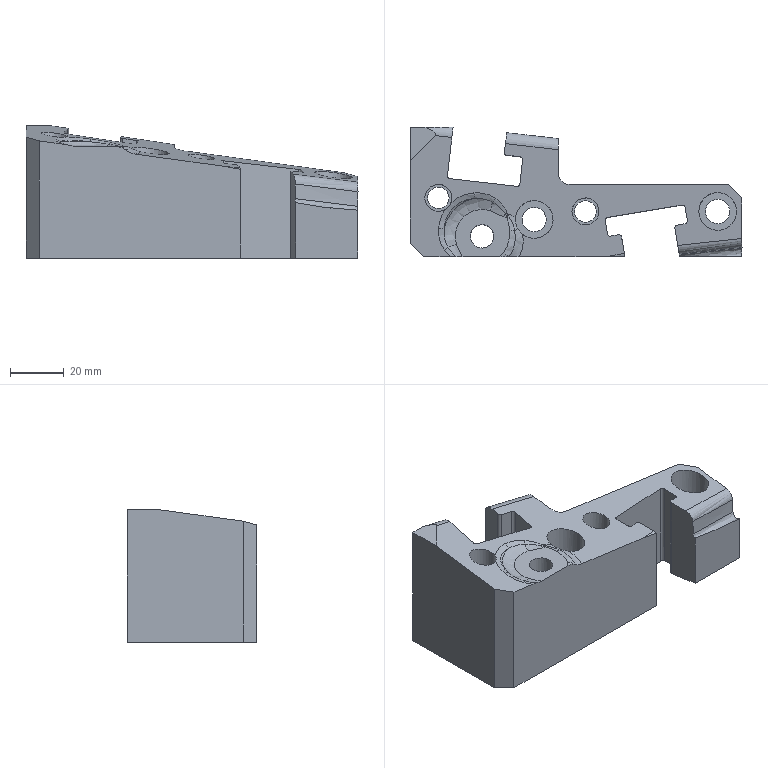Part | STEP file | gslz 2016.10.28-13_id1522_x_t | 1 solid | 75 faces | volume 122117 mm3 | plane 29 | spline 23 | cylinder 22 | other 1 | commonest cylinder face diameters 2 x10 8 x3 7.5 x2 9 x2 10 x2 14 x2